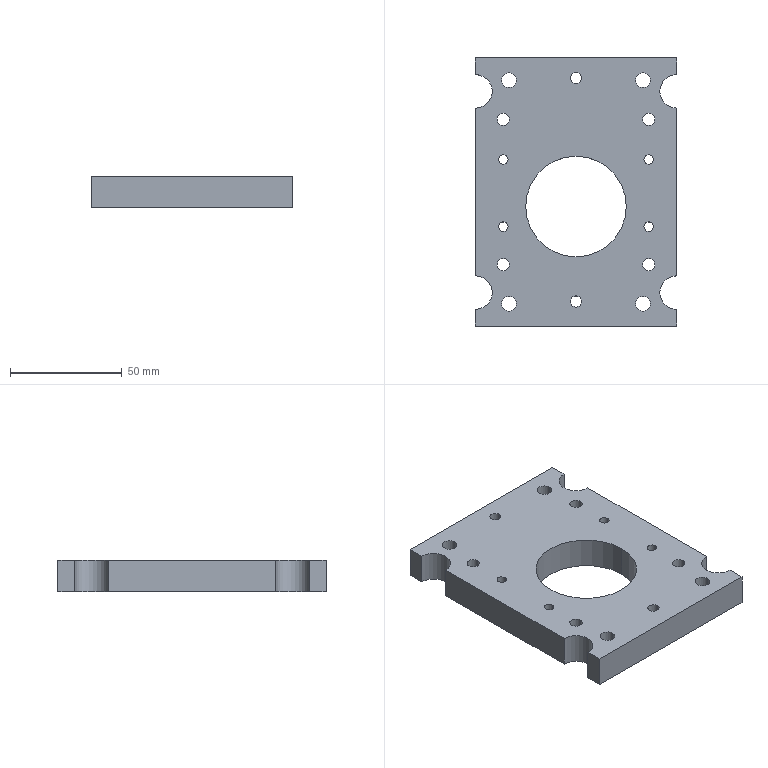Part | STEP file | bearing pad plate | 1 solid | 70 faces | box 90 x 120 x 14 mm | volume 116838 mm3 | cylinder 52 | plane 18 | commonest cylinder face diameters 4.2 x8 5.5 x8 6.6 x8 9 x8 11 x8 15 x6